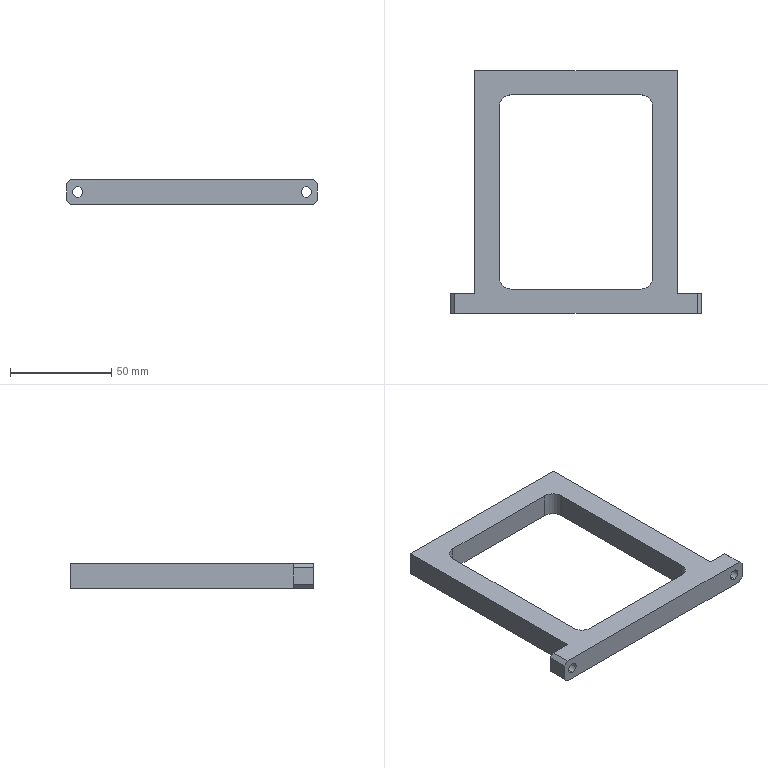Part | STEP file | QA-FC06 | 1 solid | 34 faces | box 124 x 120 x 12 mm | volume 58795 mm3 | plane 18 | cylinder 12 | cone 4 | commonest cylinder face diameters 4.2 x4 5.2 x4 12 x4